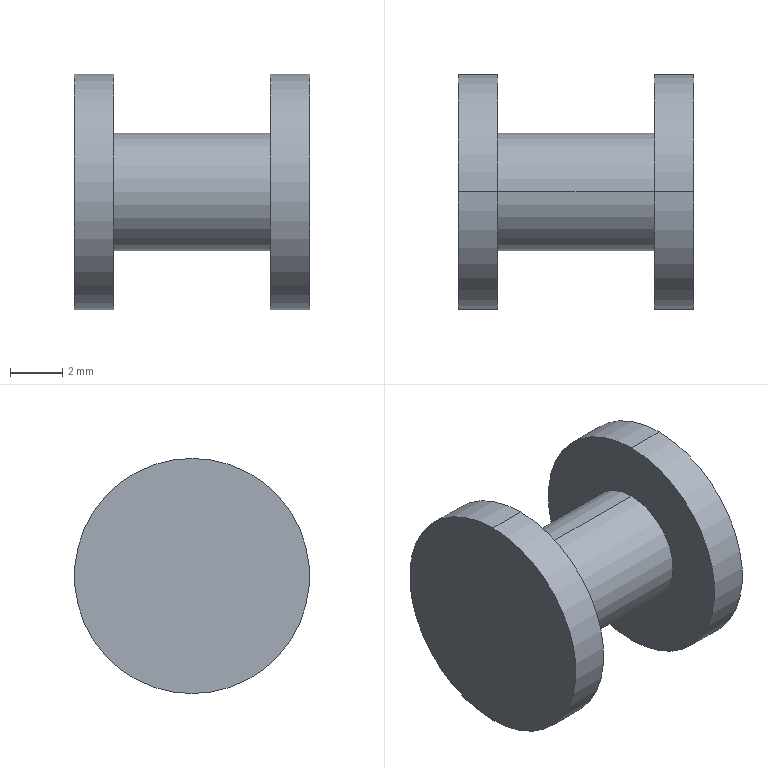Part | SolidWorks | features Revolution 1, Scale 1 | 1 solid | 10 faces | box 9 x 9 x 9 mm | volume 286.278 mm3 | cylinder 6 | plane 4 | commonest cylinder face diameters 9 x4 4.5 x2
STEP:
#1=CARTESIAN_POINT('',(3.,0.,-4.5));
#2=VERTEX_POINT('',#1);
#3=CARTESIAN_POINT('',(3.,0.,4.5));
#4=VERTEX_POINT('',#3);
#5=CARTESIAN_POINT('',(3.,0.,0.));
#6=DIRECTION('',(1.,0.,0.));
#7=DIRECTION('',(0.,0.,-1.));
#8=AXIS2_PLACEMENT_3D('',#5,#6,#7);
#9=CIRCLE('',#8,4.5);
#10=EDGE_CURVE('',#2,#4,#9,.T.);
#11=ORIENTED_EDGE('',*,*,#10,.T.);
#12=CARTESIAN_POINT('',(4.5,0.,4.5));
#13=VERTEX_POINT('',#12);
#14=CARTESIAN_POINT('',(4.5,0.,4.5));
#15=DIRECTION('',(1.,0.,0.));
#16=VECTOR('',#15,1000.);
#17=LINE('',#14,#16);
#18=EDGE_CURVE('',#4,#13,#17,.T.);
#19=ORIENTED_EDGE('',*,*,#18,.T.);
#20=CARTESIAN_POINT('',(4.5,0.,-4.5));
#21=VERTEX_POINT('',#20);
#22=CARTESIAN_POINT('',(4.5,0.,0.));
#23=DIRECTION('',(1.,0.,0.));
#24=DIRECTION('',(0.,0.,-1.));
#25=AXIS2_PLACEMENT_3D('',#22,#23,#24);
#26=CIRCLE('',#25,4.5);
#27=EDGE_CURVE('',#21,#13,#26,.T.);
#28=ORIENTED_EDGE('',*,*,#27,.F.);
#29=CARTESIAN_POINT('',(4.5,0.,-4.5));
#30=DIRECTION('',(1.,0.,0.));
#31=VECTOR('',#30,1000.);
#32=LINE('',#29,#31);
#33=EDGE_CURVE('',#2,#21,#32,.T.);
#34=ORIENTED_EDGE('',*,*,#33,.F.);
#35=EDGE_LOOP('',(#11,#19,#28,#34));
#36=FACE_OUTER_BOUND('',#35,.T.);
#37=CARTESIAN_POINT('',(4.5,0.,0.));
#38=DIRECTION('',(1.,0.,0.));
#39=DIRECTION('',(0.,0.,-1.));
#40=AXIS2_PLACEMENT_3D('',#37,#38,#39);
#41=CYLINDRICAL_SURFACE('',#40,4.5);
#42=ADVANCED_FACE('',(#36),#41,.T.);
#43=CARTESIAN_POINT('',(-4.5,0.,-4.5));
#44=VERTEX_POINT('',#43);
#45=CARTESIAN_POINT('',(-4.5,0.,4.5));
#46=VERTEX_POINT('',#45);
#47=CARTESIAN_POINT('',(-4.5,0.,0.));
#48=DIRECTION('',(1.,0.,0.));
#49=DIRECTION('',(0.,0.,-1.));
#50=AXIS2_PLACEMENT_3D('',#47,#48,#49);
#51=CIRCLE('',#50,4.5);
#52=EDGE_CURVE('',#44,#46,#51,.T.);
#53=ORIENTED_EDGE('',*,*,#52,.T.);
#54=CARTESIAN_POINT('',(-3.,0.,4.5));
#55=VERTEX_POINT('',#54);
#56=CARTESIAN_POINT('',(4.5,0.,4.5));
#57=DIRECTION('',(1.,0.,0.));
#58=VECTOR('',#57,1000.);
#59=LINE('',#56,#58);
#60=EDGE_CURVE('',#46,#55,#59,.T.);
#61=ORIENTED_EDGE('',*,*,#60,.T.);
#62=CARTESIAN_POINT('',(-3.,0.,-4.5));
#63=VERTEX_POINT('',#62);
#64=CARTESIAN_POINT('',(-3.,0.,0.));
#65=DIRECTION('',(1.,0.,0.));
#66=DIRECTION('',(0.,0.,-1.));
#67=AXIS2_PLACEMENT_3D('',#64,#65,#66);
#68=CIRCLE('',#67,4.5);
#69=EDGE_CURVE('',#63,#55,#68,.T.);
#70=ORIENTED_EDGE('',*,*,#69,.F.);
#71=CARTESIAN_POINT('',(4.5,0.,-4.5));
#72=DIRECTION('',(1.,0.,0.));
#73=VECTOR('',#72,1000.);
#74=LINE('',#71,#73);
#75=EDGE_CURVE('',#44,#63,#74,.T.);
#76=ORIENTED_EDGE('',*,*,#75,.F.);
#77=EDGE_LOOP('',(#53,#61,#70,#76));
#78=FACE_OUTER_BOUND('',#77,.T.);
#79=CARTESIAN_POINT('',(4.5,0.,0.));
#80=DIRECTION('',(1.,0.,0.));
#81=DIRECTION('',(0.,0.,-1.));
#82=AXIS2_PLACEMENT_3D('',#79,#80,#81);
#83=CYLINDRICAL_SURFACE('',#82,4.5);
#84=ADVANCED_FACE('',(#78),#83,.T.);
#85=CARTESIAN_POINT('',(-3.,0.,-2.25));
#86=VERTEX_POINT('',#85);
#87=CARTESIAN_POINT('',(-3.,0.,2.25));
#88=VERTEX_POINT('',#87);
#89=CARTESIAN_POINT('',(-3.,0.,0.));
#90=DIRECTION('',(1.,0.,0.));
#91=DIRECTION('',(0.,0.,-1.));
#92=AXIS2_PLACEMENT_3D('',#89,#90,#91);
#93=CIRCLE('',#92,2.25);
#94=EDGE_CURVE('',#86,#88,#93,.T.);
#95=ORIENTED_EDGE('',*,*,#94,.T.);
#96=CARTESIAN_POINT('',(3.,0.,2.25));
#97=VERTEX_POINT('',#96);
#98=CARTESIAN_POINT('',(4.5,0.,2.25));
#99=DIRECTION('',(1.,0.,0.));
#100=VECTOR('',#99,1000.);
#101=LINE('',#98,#100);
#102=EDGE_CURVE('',#88,#97,#101,.T.);
#103=ORIENTED_EDGE('',*,*,#102,.T.);
#104=CARTESIAN_POINT('',(3.,0.,-2.25));
#105=VERTEX_POINT('',#104);
#106=CARTESIAN_POINT('',(3.,0.,0.));
#107=DIRECTION('',(1.,0.,0.));
#108=DIRECTION('',(0.,0.,-1.));
#109=AXIS2_PLACEMENT_3D('',#106,#107,#108);
#110=CIRCLE('',#109,2.25);
#111=EDGE_CURVE('',#105,#97,#110,.T.);
#112=ORIENTED_EDGE('',*,*,#111,.F.);
#113=CARTESIAN_POINT('',(4.5,0.,-2.25));
#114=DIRECTION('',(1.,0.,0.));
#115=VECTOR('',#114,1000.);
#116=LINE('',#113,#115);
#117=EDGE_CURVE('',#86,#105,#116,.T.);
#118=ORIENTED_EDGE('',*,*,#117,.F.);
#119=EDGE_LOOP('',(#95,#103,#112,#118));
#120=FACE_OUTER_BOUND('',#119,.T.);
#121=CARTESIAN_POINT('',(4.5,0.,0.));
#122=DIRECTION('',(1.,0.,0.));
#123=DIRECTION('',(0.,0.,-1.));
#124=AXIS2_PLACEMENT_3D('',#121,#122,#123);
#125=CYLINDRICAL_SURFACE('',#124,2.25);
#126=ADVANCED_FACE('',(#120),#125,.T.);
#127=ORIENTED_EDGE('',*,*,#102,.F.);
#128=CARTESIAN_POINT('',(-3.,0.,0.));
#129=DIRECTION('',(1.,0.,0.));
#130=DIRECTION('',(0.,0.,-1.));
#131=AXIS2_PLACEMENT_3D('',#128,#129,#130);
#132=CIRCLE('',#131,2.25);
#133=EDGE_CURVE('',#88,#86,#132,.T.);
#134=ORIENTED_EDGE('',*,*,#133,.T.);
#135=ORIENTED_EDGE('',*,*,#117,.T.);
#136=CARTESIAN_POINT('',(3.,0.,0.));
#137=DIRECTION('',(1.,0.,0.));
#138=DIRECTION('',(0.,0.,-1.));
#139=AXIS2_PLACEMENT_3D('',#136,#137,#138);
#140=CIRCLE('',#139,2.25);
#141=EDGE_CURVE('',#97,#105,#140,.T.);
#142=ORIENTED_EDGE('',*,*,#141,.F.);
#143=EDGE_LOOP('',(#127,#134,#135,#142));
#144=FACE_OUTER_BOUND('',#143,.T.);
#145=CARTESIAN_POINT('',(4.5,0.,0.));
#146=DIRECTION('',(1.,0.,0.));
#147=DIRECTION('',(0.,0.,-1.));
#148=AXIS2_PLACEMENT_3D('',#145,#146,#147);
#149=CYLINDRICAL_SURFACE('',#148,2.25);
#150=ADVANCED_FACE('',(#144),#149,.T.);
#151=ORIENTED_EDGE('',*,*,#94,.F.);
#152=ORIENTED_EDGE('',*,*,#133,.F.);
#153=EDGE_LOOP('',(#151,#152));
#154=FACE_BOUND('',#153,.T.);
#155=ORIENTED_EDGE('',*,*,#69,.T.);
#156=CARTESIAN_POINT('',(-3.,0.,0.));
#157=DIRECTION('',(1.,0.,0.));
#158=DIRECTION('',(0.,0.,-1.));
#159=AXIS2_PLACEMENT_3D('',#156,#157,#158);
#160=CIRCLE('',#159,4.5);
#161=EDGE_CURVE('',#55,#63,#160,.T.);
#162=ORIENTED_EDGE('',*,*,#161,.T.);
#163=EDGE_LOOP('',(#155,#162));
#164=FACE_OUTER_BOUND('',#163,.T.);
#165=CARTESIAN_POINT('',(-3.,-4.5,0.));
#166=DIRECTION('',(-1.,0.,0.));
#167=DIRECTION('',(0.,0.,1.));
#168=AXIS2_PLACEMENT_3D('',#165,#166,#167);
#169=PLANE('',#168);
#170=ADVANCED_FACE('',(#154,#164),#169,.F.);
#171=ORIENTED_EDGE('',*,*,#60,.F.);
#172=CARTESIAN_POINT('',(-4.5,0.,0.));
#173=DIRECTION('',(1.,0.,0.));
#174=DIRECTION('',(0.,0.,-1.));
#175=AXIS2_PLACEMENT_3D('',#172,#173,#174);
#176=CIRCLE('',#175,4.5);
#177=EDGE_CURVE('',#46,#44,#176,.T.);
#178=ORIENTED_EDGE('',*,*,#177,.T.);
#179=ORIENTED_EDGE('',*,*,#75,.T.);
#180=ORIENTED_EDGE('',*,*,#161,.F.);
#181=EDGE_LOOP('',(#171,#178,#179,#180));
#182=FACE_OUTER_BOUND('',#181,.T.);
#183=CARTESIAN_POINT('',(4.5,0.,0.));
#184=DIRECTION('',(1.,0.,0.));
#185=DIRECTION('',(0.,0.,-1.));
#186=AXIS2_PLACEMENT_3D('',#183,#184,#185);
#187=CYLINDRICAL_SURFACE('',#186,4.5);
#188=ADVANCED_FACE('',(#182),#187,.T.);
#189=ORIENTED_EDGE('',*,*,#52,.F.);
#190=ORIENTED_EDGE('',*,*,#177,.F.);
#191=EDGE_LOOP('',(#189,#190));
#192=FACE_OUTER_BOUND('',#191,.T.);
#193=CARTESIAN_POINT('',(-4.5,0.,0.));
#194=DIRECTION('',(1.,0.,0.));
#195=DIRECTION('',(0.,0.,-1.));
#196=AXIS2_PLACEMENT_3D('',#193,#194,#195);
#197=PLANE('',#196);
#198=ADVANCED_FACE('',(#192),#197,.F.);
#199=ORIENTED_EDGE('',*,*,#27,.T.);
#200=CARTESIAN_POINT('',(4.5,0.,0.));
#201=DIRECTION('',(1.,0.,0.));
#202=DIRECTION('',(0.,0.,-1.));
#203=AXIS2_PLACEMENT_3D('',#200,#201,#202);
#204=CIRCLE('',#203,4.5);
#205=EDGE_CURVE('',#13,#21,#204,.T.);
#206=ORIENTED_EDGE('',*,*,#205,.T.);
#207=EDGE_LOOP('',(#199,#206));
#208=FACE_OUTER_BOUND('',#207,.T.);
#209=CARTESIAN_POINT('',(4.5,-4.5,0.));
#210=DIRECTION('',(-1.,0.,0.));
#211=DIRECTION('',(0.,0.,1.));
#212=AXIS2_PLACEMENT_3D('',#209,#210,#211);
#213=PLANE('',#212);
#214=ADVANCED_FACE('',(#208),#213,.F.);
#215=ORIENTED_EDGE('',*,*,#18,.F.);
#216=CARTESIAN_POINT('',(3.,0.,0.));
#217=DIRECTION('',(1.,0.,0.));
#218=DIRECTION('',(0.,0.,-1.));
#219=AXIS2_PLACEMENT_3D('',#216,#217,#218);
#220=CIRCLE('',#219,4.5);
#221=EDGE_CURVE('',#4,#2,#220,.T.);
#222=ORIENTED_EDGE('',*,*,#221,.T.);
#223=ORIENTED_EDGE('',*,*,#33,.T.);
#224=ORIENTED_EDGE('',*,*,#205,.F.);
#225=EDGE_LOOP('',(#215,#222,#223,#224));
#226=FACE_OUTER_BOUND('',#225,.T.);
#227=CARTESIAN_POINT('',(4.5,0.,0.));
#228=DIRECTION('',(1.,0.,0.));
#229=DIRECTION('',(0.,0.,-1.));
#230=AXIS2_PLACEMENT_3D('',#227,#228,#229);
#231=CYLINDRICAL_SURFACE('',#230,4.5);
#232=ADVANCED_FACE('',(#226),#231,.T.);
#233=ORIENTED_EDGE('',*,*,#10,.F.);
#234=ORIENTED_EDGE('',*,*,#221,.F.);
#235=EDGE_LOOP('',(#233,#234));
#236=FACE_OUTER_BOUND('',#235,.T.);
#237=ORIENTED_EDGE('',*,*,#111,.T.);
#238=ORIENTED_EDGE('',*,*,#141,.T.);
#239=EDGE_LOOP('',(#237,#238));
#240=FACE_BOUND('',#239,.T.);
#241=CARTESIAN_POINT('',(3.,-2.25,0.));
#242=DIRECTION('',(1.,0.,0.));
#243=DIRECTION('',(0.,0.,-1.));
#244=AXIS2_PLACEMENT_3D('',#241,#242,#243);
#245=PLANE('',#244);
#246=ADVANCED_FACE('',(#236,#240),#245,.F.);
#247=CLOSED_SHELL('',(#42,#84,#126,#150,#170,#188,#198,#214,#232,#246));
#248=MANIFOLD_SOLID_BREP('',#247);
#249=CARTESIAN_POINT('',(0.,0.,0.));
#250=DIRECTION('',(0.,0.,1.));
#251=DIRECTION('',(1.,0.,0.));
#252=AXIS2_PLACEMENT_3D('',#249,#250,#251);
#253=(LENGTH_UNIT()NAMED_UNIT(*)SI_UNIT(.MILLI.,.METRE.));
#254=UNCERTAINTY_MEASURE_WITH_UNIT(LENGTH_MEASURE(0.00001),#253,'','');
#255=(NAMED_UNIT(*)PLANE_ANGLE_UNIT()SI_UNIT($,.RADIAN.));
#256=(NAMED_UNIT(*)SI_UNIT($,.STERADIAN.)SOLID_ANGLE_UNIT());
#257=(GEOMETRIC_REPRESENTATION_CONTEXT(3)GLOBAL_UNCERTAINTY_ASSIGNED_CONTEXT((#254))GLOBAL_UNIT_ASSIGNED_CONTEXT((#253,#255,#256))REPRESENTATION_CONTEXT('',''));
#258=ADVANCED_BREP_SHAPE_REPRESENTATION('',(#248,#252),#257);